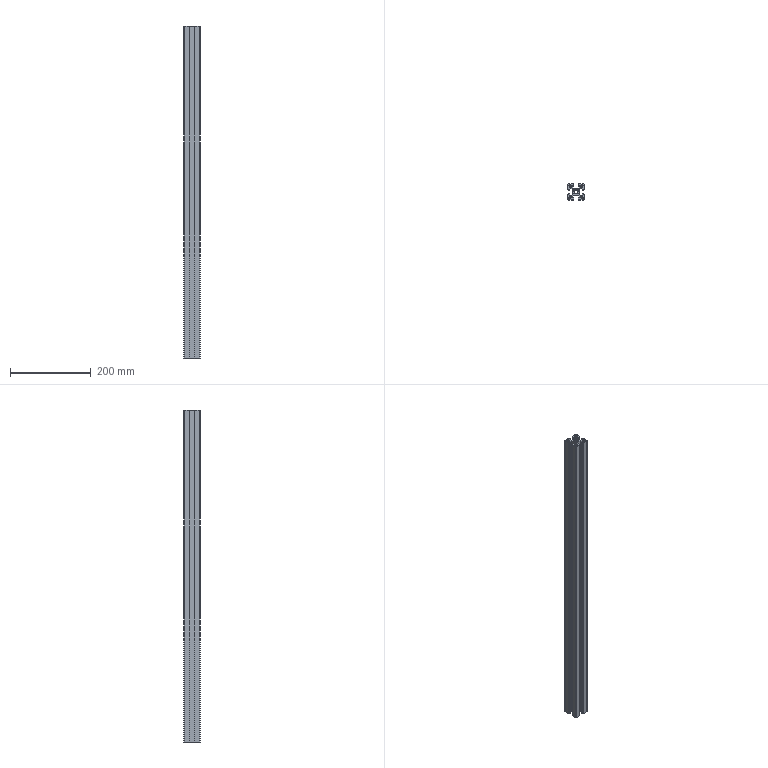Part | SolidWorks | features BaseBody 1 | 1 solid | 125 faces | box 40 x 40 x 820 mm | volume 575203 mm3 | plane 74 | cylinder 51 | commonest cylinder face diameters 2 x24 1.5 x10 5 x8 10.2 x5 4 x4